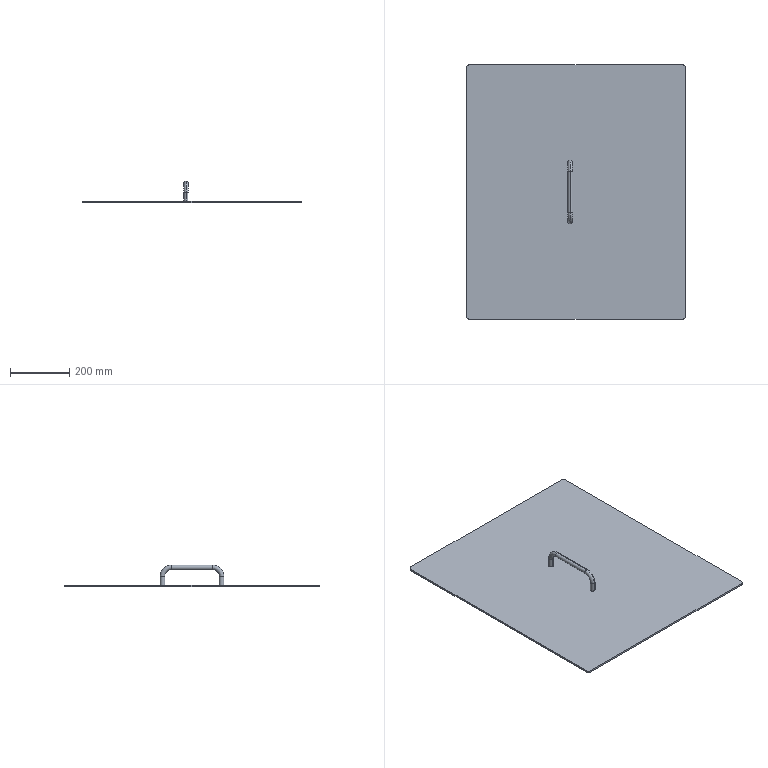Part | STEP file | Door_Default<As machined> | 6 solids | 30 faces | box 740 x 860 x 74 mm | volume 3877047 mm3 | plane 16 | cylinder 10 | torus 4 | commonest cylinder face diameters 16 x6 20 x4